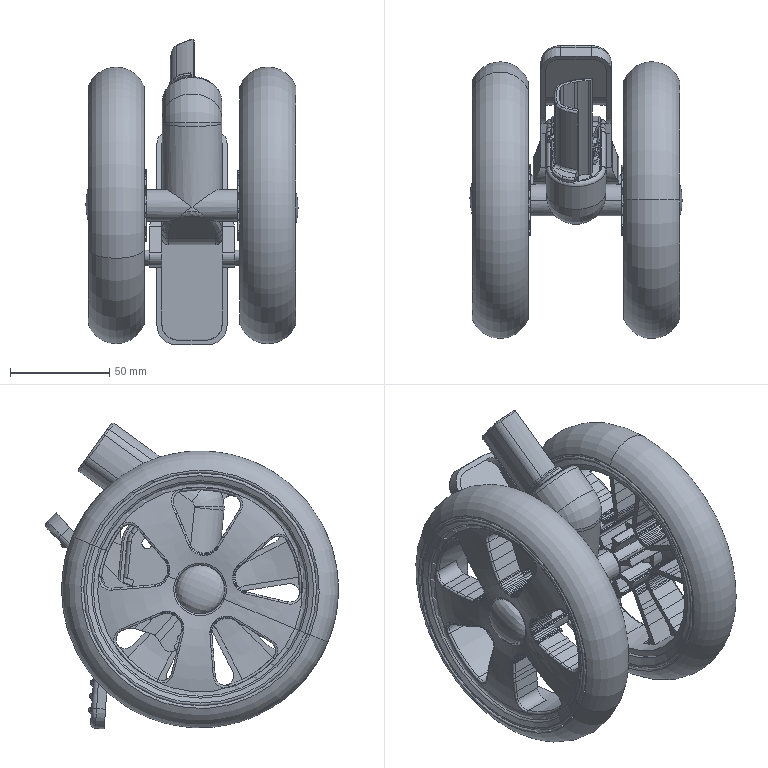Part | SolidWorks | 10 solids | 1888 faces | box 107.069 x 147.864 x 154.401 mm | volume 436546 mm3 | spline 926 | cylinder 500 | plane 260 | torus 136 | cone 52 | sphere 14 | commonest cylinder face diameters 1 x80 4 x48 3 x32 2 x28 10 x28 7 x26